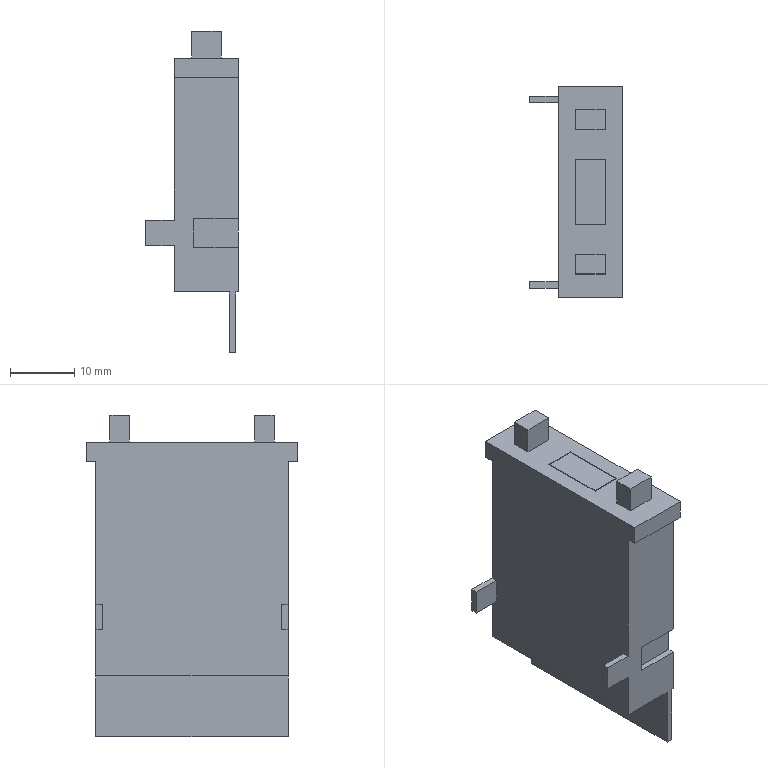Part | STEP file | A7PH_206_BASE | 1 solid | 50 faces | box 14.5 x 33 x 50.2 mm | volume 11412 mm3 | plane 50
STEP:
#1=CARTESIAN_POINT('',(-10.,-14.,-26.3));
#2=VERTEX_POINT('',#1);
#3=CARTESIAN_POINT('',(-10.,-15.,-26.3));
#4=VERTEX_POINT('',#3);
#5=CARTESIAN_POINT('',(-10.,-14.,-26.3));
#6=DIRECTION('',(0.,-1.,0.));
#7=VECTOR('',#6,1000.);
#8=LINE('',#5,#7);
#9=EDGE_CURVE('',#2,#4,#8,.T.);
#10=ORIENTED_EDGE('',*,*,#9,.F.);
#11=CARTESIAN_POINT('',(-10.,-14.,-22.3));
#12=VERTEX_POINT('',#11);
#13=CARTESIAN_POINT('',(-10.,-14.,-26.3));
#14=DIRECTION('',(0.,0.,-1.));
#15=VECTOR('',#14,1000.);
#16=LINE('',#13,#15);
#17=EDGE_CURVE('',#12,#2,#16,.T.);
#18=ORIENTED_EDGE('',*,*,#17,.F.);
#19=CARTESIAN_POINT('',(-10.,-15.,-22.3));
#20=VERTEX_POINT('',#19);
#21=CARTESIAN_POINT('',(-10.,-14.,-22.3));
#22=DIRECTION('',(0.,1.,0.));
#23=VECTOR('',#22,1000.);
#24=LINE('',#21,#23);
#25=EDGE_CURVE('',#20,#12,#24,.T.);
#26=ORIENTED_EDGE('',*,*,#25,.F.);
#27=CARTESIAN_POINT('',(-10.,-15.,0.));
#28=VERTEX_POINT('',#27);
#29=CARTESIAN_POINT('',(-10.,-15.,0.));
#30=DIRECTION('',(0.,0.,-1.));
#31=VECTOR('',#30,1000.);
#32=LINE('',#29,#31);
#33=EDGE_CURVE('',#28,#20,#32,.T.);
#34=ORIENTED_EDGE('',*,*,#33,.F.);
#35=CARTESIAN_POINT('',(-10.,-16.5,0.));
#36=VERTEX_POINT('',#35);
#37=CARTESIAN_POINT('',(-10.,-16.5,0.));
#38=DIRECTION('',(0.,1.,0.));
#39=VECTOR('',#38,1000.);
#40=LINE('',#37,#39);
#41=EDGE_CURVE('',#36,#28,#40,.T.);
#42=ORIENTED_EDGE('',*,*,#41,.F.);
#43=CARTESIAN_POINT('',(-10.,-16.5,3.));
#44=VERTEX_POINT('',#43);
#45=CARTESIAN_POINT('',(-10.,-16.5,3.));
#46=DIRECTION('',(0.,0.,-1.));
#47=VECTOR('',#46,1000.);
#48=LINE('',#45,#47);
#49=EDGE_CURVE('',#44,#36,#48,.T.);
#50=ORIENTED_EDGE('',*,*,#49,.F.);
#51=CARTESIAN_POINT('',(-10.,16.5,3.));
#52=VERTEX_POINT('',#51);
#53=CARTESIAN_POINT('',(-10.,16.5,3.));
#54=DIRECTION('',(0.,-1.,0.));
#55=VECTOR('',#54,1000.);
#56=LINE('',#53,#55);
#57=EDGE_CURVE('',#52,#44,#56,.T.);
#58=ORIENTED_EDGE('',*,*,#57,.F.);
#59=CARTESIAN_POINT('',(-10.,16.5,0.));
#60=VERTEX_POINT('',#59);
#61=CARTESIAN_POINT('',(-10.,16.5,0.));
#62=DIRECTION('',(0.,0.,1.));
#63=VECTOR('',#62,1000.);
#64=LINE('',#61,#63);
#65=EDGE_CURVE('',#60,#52,#64,.T.);
#66=ORIENTED_EDGE('',*,*,#65,.F.);
#67=CARTESIAN_POINT('',(-10.,15.,0.));
#68=VERTEX_POINT('',#67);
#69=CARTESIAN_POINT('',(-10.,15.,0.));
#70=DIRECTION('',(0.,1.,0.));
#71=VECTOR('',#70,1000.);
#72=LINE('',#69,#71);
#73=EDGE_CURVE('',#68,#60,#72,.T.);
#74=ORIENTED_EDGE('',*,*,#73,.F.);
#75=CARTESIAN_POINT('',(-10.,15.,-22.3));
#76=VERTEX_POINT('',#75);
#77=CARTESIAN_POINT('',(-10.,15.,0.));
#78=DIRECTION('',(0.,0.,1.));
#79=VECTOR('',#78,1000.);
#80=LINE('',#77,#79);
#81=EDGE_CURVE('',#76,#68,#80,.T.);
#82=ORIENTED_EDGE('',*,*,#81,.F.);
#83=CARTESIAN_POINT('',(-10.,14.,-22.3));
#84=VERTEX_POINT('',#83);
#85=CARTESIAN_POINT('',(-10.,15.,-22.3));
#86=DIRECTION('',(0.,1.,0.));
#87=VECTOR('',#86,1000.);
#88=LINE('',#85,#87);
#89=EDGE_CURVE('',#84,#76,#88,.T.);
#90=ORIENTED_EDGE('',*,*,#89,.F.);
#91=CARTESIAN_POINT('',(-10.,14.,-26.3));
#92=VERTEX_POINT('',#91);
#93=CARTESIAN_POINT('',(-10.,14.,-26.3));
#94=DIRECTION('',(0.,0.,1.));
#95=VECTOR('',#94,1000.);
#96=LINE('',#93,#95);
#97=EDGE_CURVE('',#92,#84,#96,.T.);
#98=ORIENTED_EDGE('',*,*,#97,.F.);
#99=CARTESIAN_POINT('',(-10.,15.,-26.3));
#100=VERTEX_POINT('',#99);
#101=CARTESIAN_POINT('',(-10.,15.,-26.3));
#102=DIRECTION('',(0.,-1.,0.));
#103=VECTOR('',#102,1000.);
#104=LINE('',#101,#103);
#105=EDGE_CURVE('',#100,#92,#104,.T.);
#106=ORIENTED_EDGE('',*,*,#105,.F.);
#107=CARTESIAN_POINT('',(-10.,15.,-33.5));
#108=VERTEX_POINT('',#107);
#109=CARTESIAN_POINT('',(-10.,15.,0.));
#110=DIRECTION('',(0.,0.,1.));
#111=VECTOR('',#110,1000.);
#112=LINE('',#109,#111);
#113=EDGE_CURVE('',#108,#100,#112,.T.);
#114=ORIENTED_EDGE('',*,*,#113,.F.);
#115=CARTESIAN_POINT('',(-10.,-15.,-33.5));
#116=VERTEX_POINT('',#115);
#117=CARTESIAN_POINT('',(-10.,15.,-33.5));
#118=DIRECTION('',(0.,1.,0.));
#119=VECTOR('',#118,1000.);
#120=LINE('',#117,#119);
#121=EDGE_CURVE('',#116,#108,#120,.T.);
#122=ORIENTED_EDGE('',*,*,#121,.F.);
#123=CARTESIAN_POINT('',(-10.,-15.,0.));
#124=DIRECTION('',(0.,0.,-1.));
#125=VECTOR('',#124,1000.);
#126=LINE('',#123,#125);
#127=EDGE_CURVE('',#4,#116,#126,.T.);
#128=ORIENTED_EDGE('',*,*,#127,.F.);
#129=EDGE_LOOP('',(#10,#18,#26,#34,#42,#50,#58,#66,#74,#82,#90,#98,#106,#114,#122,#128));
#130=FACE_OUTER_BOUND('',#129,.T.);
#131=CARTESIAN_POINT('',(-10.,16.5,0.));
#132=DIRECTION('',(1.,0.,0.));
#133=DIRECTION('',(0.,0.,-1.));
#134=AXIS2_PLACEMENT_3D('',#131,#132,#133);
#135=PLANE('',#134);
#136=ADVANCED_FACE('',(#130),#135,.F.);
#137=CARTESIAN_POINT('',(-1.4,15.,-33.5));
#138=VERTEX_POINT('',#137);
#139=CARTESIAN_POINT('',(-10.,15.,-33.5));
#140=DIRECTION('',(1.,0.,0.));
#141=VECTOR('',#140,1000.);
#142=LINE('',#139,#141);
#143=EDGE_CURVE('',#108,#138,#142,.T.);
#144=ORIENTED_EDGE('',*,*,#143,.T.);
#145=CARTESIAN_POINT('',(-1.4,-15.,-33.5));
#146=VERTEX_POINT('',#145);
#147=CARTESIAN_POINT('',(-1.4,24.552,-33.5));
#148=DIRECTION('',(0.,-1.,0.));
#149=VECTOR('',#148,1000.);
#150=LINE('',#147,#149);
#151=EDGE_CURVE('',#138,#146,#150,.T.);
#152=ORIENTED_EDGE('',*,*,#151,.T.);
#153=CARTESIAN_POINT('',(-10.,-15.,-33.5));
#154=DIRECTION('',(1.,0.,0.));
#155=VECTOR('',#154,1000.);
#156=LINE('',#153,#155);
#157=EDGE_CURVE('',#116,#146,#156,.T.);
#158=ORIENTED_EDGE('',*,*,#157,.F.);
#159=ORIENTED_EDGE('',*,*,#121,.T.);
#160=EDGE_LOOP('',(#144,#152,#158,#159));
#161=FACE_OUTER_BOUND('',#160,.T.);
#162=CARTESIAN_POINT('',(-10.,15.,-33.5));
#163=DIRECTION('',(0.,0.,-1.));
#164=DIRECTION('',(-1.,0.,0.));
#165=AXIS2_PLACEMENT_3D('',#162,#163,#164);
#166=PLANE('',#165);
#167=ADVANCED_FACE('',(#161),#166,.T.);
#168=CARTESIAN_POINT('',(-7.4,5.1,3.));
#169=VERTEX_POINT('',#168);
#170=CARTESIAN_POINT('',(-7.4,-5.1,3.));
#171=VERTEX_POINT('',#170);
#172=CARTESIAN_POINT('',(-7.4,5.,3.));
#173=DIRECTION('',(0.,-1.,0.));
#174=VECTOR('',#173,1000.);
#175=LINE('',#172,#174);
#176=EDGE_CURVE('',#169,#171,#175,.T.);
#177=ORIENTED_EDGE('',*,*,#176,.F.);
#178=CARTESIAN_POINT('',(-2.6,5.1,3.));
#179=VERTEX_POINT('',#178);
#180=CARTESIAN_POINT('',(-7.3,5.1,3.));
#181=DIRECTION('',(-1.,0.,0.));
#182=VECTOR('',#181,1000.);
#183=LINE('',#180,#182);
#184=EDGE_CURVE('',#179,#169,#183,.T.);
#185=ORIENTED_EDGE('',*,*,#184,.F.);
#186=CARTESIAN_POINT('',(-2.6,-5.1,3.));
#187=VERTEX_POINT('',#186);
#188=CARTESIAN_POINT('',(-2.6,5.,3.));
#189=DIRECTION('',(0.,1.,0.));
#190=VECTOR('',#189,1000.);
#191=LINE('',#188,#190);
#192=EDGE_CURVE('',#187,#179,#191,.T.);
#193=ORIENTED_EDGE('',*,*,#192,.F.);
#194=CARTESIAN_POINT('',(-7.3,-5.1,3.));
#195=DIRECTION('',(1.,0.,0.));
#196=VECTOR('',#195,1000.);
#197=LINE('',#194,#196);
#198=EDGE_CURVE('',#171,#187,#197,.T.);
#199=ORIENTED_EDGE('',*,*,#198,.F.);
#200=EDGE_LOOP('',(#177,#185,#193,#199));
#201=FACE_BOUND('',#200,.T.);
#202=CARTESIAN_POINT('',(-7.3,-12.8,3.));
#203=VERTEX_POINT('',#202);
#204=CARTESIAN_POINT('',(-7.3,-9.8,3.));
#205=VERTEX_POINT('',#204);
#206=CARTESIAN_POINT('',(-7.3,-12.8,3.));
#207=DIRECTION('',(0.,1.,0.));
#208=VECTOR('',#207,1000.);
#209=LINE('',#206,#208);
#210=EDGE_CURVE('',#203,#205,#209,.T.);
#211=ORIENTED_EDGE('',*,*,#210,.T.);
#212=CARTESIAN_POINT('',(-2.7,-9.8,3.));
#213=VERTEX_POINT('',#212);
#214=CARTESIAN_POINT('',(-7.3,-9.8,3.));
#215=DIRECTION('',(1.,0.,0.));
#216=VECTOR('',#215,1000.);
#217=LINE('',#214,#216);
#218=EDGE_CURVE('',#205,#213,#217,.T.);
#219=ORIENTED_EDGE('',*,*,#218,.T.);
#220=CARTESIAN_POINT('',(-2.7,-12.8,3.));
#221=VERTEX_POINT('',#220);
#222=CARTESIAN_POINT('',(-2.7,-12.8,3.));
#223=DIRECTION('',(0.,-1.,0.));
#224=VECTOR('',#223,1000.);
#225=LINE('',#222,#224);
#226=EDGE_CURVE('',#213,#221,#225,.T.);
#227=ORIENTED_EDGE('',*,*,#226,.T.);
#228=CARTESIAN_POINT('',(-7.3,-12.8,3.));
#229=DIRECTION('',(-1.,0.,0.));
#230=VECTOR('',#229,1000.);
#231=LINE('',#228,#230);
#232=EDGE_CURVE('',#221,#203,#231,.T.);
#233=ORIENTED_EDGE('',*,*,#232,.T.);
#234=EDGE_LOOP('',(#211,#219,#227,#233));
#235=FACE_BOUND('',#234,.T.);
#236=CARTESIAN_POINT('',(0.,16.5,3.));
#237=VERTEX_POINT('',#236);
#238=CARTESIAN_POINT('',(0.,-16.5,3.));
#239=VERTEX_POINT('',#238);
#240=CARTESIAN_POINT('',(0.,16.5,3.));
#241=DIRECTION('',(0.,-1.,0.));
#242=VECTOR('',#241,1000.);
#243=LINE('',#240,#242);
#244=EDGE_CURVE('',#237,#239,#243,.T.);
#245=ORIENTED_EDGE('',*,*,#244,.F.);
#246=CARTESIAN_POINT('',(-10.,16.5,3.));
#247=DIRECTION('',(1.,0.,0.));
#248=VECTOR('',#247,1000.);
#249=LINE('',#246,#248);
#250=EDGE_CURVE('',#52,#237,#249,.T.);
#251=ORIENTED_EDGE('',*,*,#250,.F.);
#252=ORIENTED_EDGE('',*,*,#57,.T.);
#253=CARTESIAN_POINT('',(-10.,-16.5,3.));
#254=DIRECTION('',(1.,0.,0.));
#255=VECTOR('',#254,1000.);
#256=LINE('',#253,#255);
#257=EDGE_CURVE('',#44,#239,#256,.T.);
#258=ORIENTED_EDGE('',*,*,#257,.T.);
#259=EDGE_LOOP('',(#245,#251,#252,#258));
#260=FACE_OUTER_BOUND('',#259,.T.);
#261=CARTESIAN_POINT('',(-7.3,9.8,3.));
#262=VERTEX_POINT('',#261);
#263=CARTESIAN_POINT('',(-2.7,9.8,3.));
#264=VERTEX_POINT('',#263);
#265=CARTESIAN_POINT('',(-7.3,9.8,3.));
#266=DIRECTION('',(1.,0.,0.));
#267=VECTOR('',#266,1000.);
#268=LINE('',#265,#267);
#269=EDGE_CURVE('',#262,#264,#268,.T.);
#270=ORIENTED_EDGE('',*,*,#269,.F.);
#271=CARTESIAN_POINT('',(-7.3,12.8,3.));
#272=VERTEX_POINT('',#271);
#273=CARTESIAN_POINT('',(-7.3,12.8,3.));
#274=DIRECTION('',(0.,-1.,0.));
#275=VECTOR('',#274,1000.);
#276=LINE('',#273,#275);
#277=EDGE_CURVE('',#272,#262,#276,.T.);
#278=ORIENTED_EDGE('',*,*,#277,.F.);
#279=CARTESIAN_POINT('',(-2.7,12.8,3.));
#280=VERTEX_POINT('',#279);
#281=CARTESIAN_POINT('',(-7.3,12.8,3.));
#282=DIRECTION('',(-1.,0.,0.));
#283=VECTOR('',#282,1000.);
#284=LINE('',#281,#283);
#285=EDGE_CURVE('',#280,#272,#284,.T.);
#286=ORIENTED_EDGE('',*,*,#285,.F.);
#287=CARTESIAN_POINT('',(-2.7,12.8,3.));
#288=DIRECTION('',(0.,1.,0.));
#289=VECTOR('',#288,1000.);
#290=LINE('',#287,#289);
#291=EDGE_CURVE('',#264,#280,#290,.T.);
#292=ORIENTED_EDGE('',*,*,#291,.F.);
#293=EDGE_LOOP('',(#270,#278,#286,#292));
#294=FACE_BOUND('',#293,.T.);
#295=CARTESIAN_POINT('',(-10.,16.5,3.));
#296=DIRECTION('',(0.,0.,1.));
#297=DIRECTION('',(1.,0.,0.));
#298=AXIS2_PLACEMENT_3D('',#295,#296,#297);
#299=PLANE('',#298);
#300=ADVANCED_FACE('',(#201,#235,#260,#294),#299,.T.);
#301=CARTESIAN_POINT('',(0.,15.,0.));
#302=VERTEX_POINT('',#301);
#303=CARTESIAN_POINT('',(0.,16.5,0.));
#304=VERTEX_POINT('',#303);
#305=CARTESIAN_POINT('',(0.,15.,0.));
#306=DIRECTION('',(0.,1.,0.));
#307=VECTOR('',#306,1000.);
#308=LINE('',#305,#307);
#309=EDGE_CURVE('',#302,#304,#308,.T.);
#310=ORIENTED_EDGE('',*,*,#309,.F.);
#311=CARTESIAN_POINT('',(-10.,15.,0.));
#312=DIRECTION('',(1.,0.,0.));
#313=VECTOR('',#312,1000.);
#314=LINE('',#311,#313);
#315=EDGE_CURVE('',#68,#302,#314,.T.);
#316=ORIENTED_EDGE('',*,*,#315,.F.);
#317=ORIENTED_EDGE('',*,*,#73,.T.);
#318=CARTESIAN_POINT('',(-10.,16.5,0.));
#319=DIRECTION('',(1.,0.,0.));
#320=VECTOR('',#319,1000.);
#321=LINE('',#318,#320);
#322=EDGE_CURVE('',#60,#304,#321,.T.);
#323=ORIENTED_EDGE('',*,*,#322,.T.);
#324=EDGE_LOOP('',(#310,#316,#317,#323));
#325=FACE_OUTER_BOUND('',#324,.T.);
#326=CARTESIAN_POINT('',(-10.,15.,0.));
#327=DIRECTION('',(0.,0.,-1.));
#328=DIRECTION('',(0.,1.,0.));
#329=AXIS2_PLACEMENT_3D('',#326,#327,#328);
#330=PLANE('',#329);
#331=ADVANCED_FACE('',(#325),#330,.T.);
#332=CARTESIAN_POINT('',(-7.,15.,-22.1));
#333=VERTEX_POINT('',#332);
#334=CARTESIAN_POINT('',(0.,15.,-22.1));
#335=VERTEX_POINT('',#334);
#336=CARTESIAN_POINT('',(-7.,15.,-22.1));
#337=DIRECTION('',(1.,0.,0.));
#338=VECTOR('',#337,1000.);
#339=LINE('',#336,#338);
#340=EDGE_CURVE('',#333,#335,#339,.T.);
#341=ORIENTED_EDGE('',*,*,#340,.F.);
#342=CARTESIAN_POINT('',(-7.,15.,-26.5));
#343=VERTEX_POINT('',#342);
#344=CARTESIAN_POINT('',(-7.,15.,-22.1));
#345=DIRECTION('',(0.,0.,1.));
#346=VECTOR('',#345,1000.);
#347=LINE('',#344,#346);
#348=EDGE_CURVE('',#343,#333,#347,.T.);
#349=ORIENTED_EDGE('',*,*,#348,.F.);
#350=CARTESIAN_POINT('',(0.,15.,-26.5));
#351=VERTEX_POINT('',#350);
#352=CARTESIAN_POINT('',(-7.,15.,-26.5));
#353=DIRECTION('',(1.,0.,0.));
#354=VECTOR('',#353,1000.);
#355=LINE('',#352,#354);
#356=EDGE_CURVE('',#343,#351,#355,.T.);
#357=ORIENTED_EDGE('',*,*,#356,.T.);
#358=CARTESIAN_POINT('',(0.,15.,-33.5));
#359=VERTEX_POINT('',#358);
#360=CARTESIAN_POINT('',(0.,15.,0.));
#361=DIRECTION('',(0.,0.,1.));
#362=VECTOR('',#361,1000.);
#363=LINE('',#360,#362);
#364=EDGE_CURVE('',#359,#351,#363,.T.);
#365=ORIENTED_EDGE('',*,*,#364,.F.);
#366=CARTESIAN_POINT('',(-0.4,15.,-33.5));
#367=VERTEX_POINT('',#366);
#368=CARTESIAN_POINT('',(-10.,15.,-33.5));
#369=DIRECTION('',(1.,0.,0.));
#370=VECTOR('',#369,1000.);
#371=LINE('',#368,#370);
#372=EDGE_CURVE('',#367,#359,#371,.T.);
#373=ORIENTED_EDGE('',*,*,#372,.F.);
#374=CARTESIAN_POINT('',(-0.4,15.,-43.));
#375=VERTEX_POINT('',#374);
#376=CARTESIAN_POINT('',(-0.4,15.,-33.5));
#377=DIRECTION('',(0.,0.,1.));
#378=VECTOR('',#377,1000.);
#379=LINE('',#376,#378);
#380=EDGE_CURVE('',#375,#367,#379,.T.);
#381=ORIENTED_EDGE('',*,*,#380,.F.);
#382=CARTESIAN_POINT('',(-1.4,15.,-43.));
#383=VERTEX_POINT('',#382);
#384=CARTESIAN_POINT('',(-0.4,15.,-43.));
#385=DIRECTION('',(1.,0.,0.));
#386=VECTOR('',#385,1000.);
#387=LINE('',#384,#386);
#388=EDGE_CURVE('',#383,#375,#387,.T.);
#389=ORIENTED_EDGE('',*,*,#388,.F.);
#390=CARTESIAN_POINT('',(-1.4,15.,-33.5));
#391=DIRECTION('',(0.,0.,-1.));
#392=VECTOR('',#391,1000.);
#393=LINE('',#390,#392);
#394=EDGE_CURVE('',#138,#383,#393,.T.);
#395=ORIENTED_EDGE('',*,*,#394,.F.);
#396=ORIENTED_EDGE('',*,*,#143,.F.);
#397=ORIENTED_EDGE('',*,*,#113,.T.);
#398=CARTESIAN_POINT('',(-14.5,15.,-26.3));
#399=VERTEX_POINT('',#398);
#400=CARTESIAN_POINT('',(-14.5,15.,-26.3));
#401=DIRECTION('',(1.,0.,0.));
#402=VECTOR('',#401,1000.);
#403=LINE('',#400,#402);
#404=EDGE_CURVE('',#399,#100,#403,.T.);
#405=ORIENTED_EDGE('',*,*,#404,.F.);
#406=CARTESIAN_POINT('',(-14.5,15.,-22.3));
#407=VERTEX_POINT('',#406);
#408=CARTESIAN_POINT('',(-14.5,15.,-26.3));
#409=DIRECTION('',(0.,0.,-1.));
#410=VECTOR('',#409,1000.);
#411=LINE('',#408,#410);
#412=EDGE_CURVE('',#407,#399,#411,.T.);
#413=ORIENTED_EDGE('',*,*,#412,.F.);
#414=CARTESIAN_POINT('',(-14.5,15.,-22.3));
#415=DIRECTION('',(1.,0.,0.));
#416=VECTOR('',#415,1000.);
#417=LINE('',#414,#416);
#418=EDGE_CURVE('',#407,#76,#417,.T.);
#419=ORIENTED_EDGE('',*,*,#418,.T.);
#420=ORIENTED_EDGE('',*,*,#81,.T.);
#421=ORIENTED_EDGE('',*,*,#315,.T.);
#422=CARTESIAN_POINT('',(0.,15.,0.));
#423=DIRECTION('',(0.,0.,1.));
#424=VECTOR('',#423,1000.);
#425=LINE('',#422,#424);
#426=EDGE_CURVE('',#335,#302,#425,.T.);
#427=ORIENTED_EDGE('',*,*,#426,.F.);
#428=EDGE_LOOP('',(#341,#349,#357,#365,#373,#381,#389,#395,#396,#397,#405,#413,#419,#420,#421,#427));
#429=FACE_OUTER_BOUND('',#428,.T.);
#430=CARTESIAN_POINT('',(-10.,15.,0.));
#431=DIRECTION('',(0.,1.,0.));
#432=DIRECTION('',(0.,0.,1.));
#433=AXIS2_PLACEMENT_3D('',#430,#431,#432);
#434=PLANE('',#433);
#435=ADVANCED_FACE('',(#429),#434,.T.);
#436=CARTESIAN_POINT('',(-0.4,-15.,-33.5));
#437=VERTEX_POINT('',#436);
#438=CARTESIAN_POINT('',(-0.4,24.552,-33.5));
#439=DIRECTION('',(0.,-1.,0.));
#440=VECTOR('',#439,1000.);
#441=LINE('',#438,#440);
#442=EDGE_CURVE('',#367,#437,#441,.T.);
#443=ORIENTED_EDGE('',*,*,#442,.F.);
#444=ORIENTED_EDGE('',*,*,#372,.T.);
#445=CARTESIAN_POINT('',(0.,-15.,-33.5));
#446=VERTEX_POINT('',#445);
#447=CARTESIAN_POINT('',(0.,15.,-33.5));
#448=DIRECTION('',(0.,1.,0.));
#449=VECTOR('',#448,1000.);
#450=LINE('',#447,#449);
#451=EDGE_CURVE('',#446,#359,#450,.T.);
#452=ORIENTED_EDGE('',*,*,#451,.F.);
#453=CARTESIAN_POINT('',(-10.,-15.,-33.5));
#454=DIRECTION('',(1.,0.,0.));
#455=VECTOR('',#454,1000.);
#456=LINE('',#453,#455);
#457=EDGE_CURVE('',#437,#446,#456,.T.);
#458=ORIENTED_EDGE('',*,*,#457,.F.);
#459=EDGE_LOOP('',(#443,#444,#452,#458));
#460=FACE_OUTER_BOUND('',#459,.T.);
#461=CARTESIAN_POINT('',(-10.,15.,-33.5));
#462=DIRECTION('',(0.,0.,-1.));
#463=DIRECTION('',(-1.,0.,0.));
#464=AXIS2_PLACEMENT_3D('',#461,#462,#463);
#465=PLANE('',#464);
#466=ADVANCED_FACE('',(#460),#465,.T.);
#467=CARTESIAN_POINT('',(-7.,-15.,-22.1));
#468=VERTEX_POINT('',#467);
#469=CARTESIAN_POINT('',(0.,-15.,-22.1));
#470=VERTEX_POINT('',#469);
#471=CARTESIAN_POINT('',(-7.,-15.,-22.1));
#472=DIRECTION('',(1.,0.,0.));
#473=VECTOR('',#472,1000.);
#474=LINE('',#471,#473);
#475=EDGE_CURVE('',#468,#470,#474,.T.);
#476=ORIENTED_EDGE('',*,*,#475,.T.);
#477=CARTESIAN_POINT('',(0.,-15.,0.));
#478=VERTEX_POINT('',#477);
#479=CARTESIAN_POINT('',(0.,-15.,0.));
#480=DIRECTION('',(0.,0.,-1.));
#481=VECTOR('',#480,1000.);
#482=LINE('',#479,#481);
#483=EDGE_CURVE('',#478,#470,#482,.T.);
#484=ORIENTED_EDGE('',*,*,#483,.F.);
#485=CARTESIAN_POINT('',(-10.,-15.,0.));
#486=DIRECTION('',(1.,0.,0.));
#487=VECTOR('',#486,1000.);
#488=LINE('',#485,#487);
#489=EDGE_CURVE('',#28,#478,#488,.T.);
#490=ORIENTED_EDGE('',*,*,#489,.F.);
#491=ORIENTED_EDGE('',*,*,#33,.T.);
#492=CARTESIAN_POINT('',(-14.5,-15.,-22.3));
#493=VERTEX_POINT('',#492);
#494=CARTESIAN_POINT('',(-14.5,-15.,-22.3));
#495=DIRECTION('',(1.,0.,0.));
#496=VECTOR('',#495,1000.);
#497=LINE('',#494,#496);
#498=EDGE_CURVE('',#493,#20,#497,.T.);
#499=ORIENTED_EDGE('',*,*,#498,.F.);
#500=CARTESIAN_POINT('',(-14.5,-15.,-26.3));
#501=VERTEX_POINT('',#500);
#502=CARTESIAN_POINT('',(-14.5,-15.,-26.3));
#503=DIRECTION('',(0.,0.,1.));
#504=VECTOR('',#503,1000.);
#505=LINE('',#502,#504);
#506=EDGE_CURVE('',#501,#493,#505,.T.);
#507=ORIENTED_EDGE('',*,*,#506,.F.);
#508=CARTESIAN_POINT('',(-14.5,-15.,-26.3));
#509=DIRECTION('',(1.,0.,0.));
#510=VECTOR('',#509,1000.);
#511=LINE('',#508,#510);
#512=EDGE_CURVE('',#501,#4,#511,.T.);
#513=ORIENTED_EDGE('',*,*,#512,.T.);
#514=ORIENTED_EDGE('',*,*,#127,.T.);
#515=ORIENTED_EDGE('',*,*,#157,.T.);
#516=CARTESIAN_POINT('',(-1.4,-15.,-43.));
#517=VERTEX_POINT('',#516);
#518=CARTESIAN_POINT('',(-1.4,-15.,-33.5));
#519=DIRECTION('',(0.,0.,-1.));
#520=VECTOR('',#519,1000.);
#521=LINE('',#518,#520);
#522=EDGE_CURVE('',#146,#517,#521,.T.);
#523=ORIENTED_EDGE('',*,*,#522,.T.);
#524=CARTESIAN_POINT('',(-0.4,-15.,-43.));
#525=VERTEX_POINT('',#524);
#526=CARTESIAN_POINT('',(-0.4,-15.,-43.));
#527=DIRECTION('',(1.,0.,0.));
#528=VECTOR('',#527,1000.);
#529=LINE('',#526,#528);
#530=EDGE_CURVE('',#517,#525,#529,.T.);
#531=ORIENTED_EDGE('',*,*,#530,.T.);
#532=CARTESIAN_POINT('',(-0.4,-15.,-33.5));
#533=DIRECTION('',(0.,0.,1.));
#534=VECTOR('',#533,1000.);
#535=LINE('',#532,#534);
#536=EDGE_CURVE('',#525,#437,#535,.T.);
#537=ORIENTED_EDGE('',*,*,#536,.T.);
#538=ORIENTED_EDGE('',*,*,#457,.T.);
#539=CARTESIAN_POINT('',(0.,-15.,-26.5));
#540=VERTEX_POINT('',#539);
#541=CARTESIAN_POINT('',(0.,-15.,0.));
#542=DIRECTION('',(0.,0.,-1.));
#543=VECTOR('',#542,1000.);
#544=LINE('',#541,#543);
#545=EDGE_CURVE('',#540,#446,#544,.T.);
#546=ORIENTED_EDGE('',*,*,#545,.F.);
#547=CARTESIAN_POINT('',(-7.,-15.,-26.5));
#548=VERTEX_POINT('',#547);
#549=CARTESIAN_POINT('',(-7.,-15.,-26.5));
#550=DIRECTION('',(1.,0.,0.));
#551=VECTOR('',#550,1000.);
#552=LINE('',#549,#551);
#553=EDGE_CURVE('',#548,#540,#552,.T.);
#554=ORIENTED_EDGE('',*,*,#553,.F.);
#555=CARTESIAN_POINT('',(-7.,-15.,-22.1));
#556=DIRECTION('',(0.,0.,-1.));
#557=VECTOR('',#556,1000.);
#558=LINE('',#555,#557);
#559=EDGE_CURVE('',#468,#548,#558,.T.);
#560=ORIENTED_EDGE('',*,*,#559,.F.);
#561=EDGE_LOOP('',(#476,#484,#490,#491,#499,#507,#513,#514,#515,#523,#531,#537,#538,#546,#554,#560));
#562=FACE_OUTER_BOUND('',#561,.T.);
#563=CARTESIAN_POINT('',(-10.,-15.,0.));
#564=DIRECTION('',(0.,-1.,0.));
#565=DIRECTION('',(0.,0.,-1.));
#566=AXIS2_PLACEMENT_3D('',#563,#564,#565);
#567=PLANE('',#566);
#568=ADVANCED_FACE('',(#562),#567,.T.);
#569=CARTESIAN_POINT('',(0.,-16.5,0.));
#570=VERTEX_POINT('',#569);
#571=CARTESIAN_POINT('',(0.,-16.5,0.));
#572=DIRECTION('',(0.,1.,0.));
#573=VECTOR('',#572,1000.);
#574=LINE('',#571,#573);
#575=EDGE_CURVE('',#570,#478,#574,.T.);
#576=ORIENTED_EDGE('',*,*,#575,.F.);
#577=CARTESIAN_POINT('',(-10.,-16.5,0.));
#578=DIRECTION('',(1.,0.,0.));
#579=VECTOR('',#578,1000.);
#580=LINE('',#577,#579);
#581=EDGE_CURVE('',#36,#570,#580,.T.);
#582=ORIENTED_EDGE('',*,*,#581,.F.);
#583=ORIENTED_EDGE('',*,*,#41,.T.);
#584=ORIENTED_EDGE('',*,*,#489,.T.);
#585=EDGE_LOOP('',(#576,#582,#583,#584));
#586=FACE_OUTER_BOUND('',#585,.T.);
#587=CARTESIAN_POINT('',(-10.,-16.5,0.));
#588=DIRECTION('',(0.,0.,-1.));
#589=DIRECTION('',(-1.,0.,0.));
#590=AXIS2_PLACEMENT_3D('',#587,#588,#589);
#591=PLANE('',#590);
#592=ADVANCED_FACE('',(#586),#591,.T.);
#593=CARTESIAN_POINT('',(0.,-16.5,3.));
#594=DIRECTION('',(0.,0.,-1.));
#595=VECTOR('',#594,1000.);
#596=LINE('',#593,#595);
#597=EDGE_CURVE('',#239,#570,#596,.T.);
#598=ORIENTED_EDGE('',*,*,#597,.F.);
#599=ORIENTED_EDGE('',*,*,#257,.F.);
#600=ORIENTED_EDGE('',*,*,#49,.T.);
#601=ORIENTED_EDGE('',*,*,#581,.T.);
#602=EDGE_LOOP('',(#598,#599,#600,#601));
#603=FACE_OUTER_BOUND('',#602,.T.);
#604=CARTESIAN_POINT('',(-10.,-16.5,3.));
#605=DIRECTION('',(0.,-1.,0.));
#606=DIRECTION('',(0.,0.,-1.));
#607=AXIS2_PLACEMENT_3D('',#604,#605,#606);
#608=PLANE('',#607);
#609=ADVANCED_FACE('',(#603),#608,.T.);
#610=CARTESIAN_POINT('',(0.,16.5,0.));
#611=DIRECTION('',(0.,0.,1.));
#612=VECTOR('',#611,1000.);
#613=LINE('',#610,#612);
#614=EDGE_CURVE('',#304,#237,#613,.T.);
#615=ORIENTED_EDGE('',*,*,#614,.F.);
#616=ORIENTED_EDGE('',*,*,#322,.F.);
#617=ORIENTED_EDGE('',*,*,#65,.T.);
#618=ORIENTED_EDGE('',*,*,#250,.T.);
#619=EDGE_LOOP('',(#615,#616,#617,#618));
#620=FACE_OUTER_BOUND('',#619,.T.);
#621=CARTESIAN_POINT('',(-10.,16.5,0.));
#622=DIRECTION('',(0.,1.,0.));
#623=DIRECTION('',(0.,0.,1.));
#624=AXIS2_PLACEMENT_3D('',#621,#622,#623);
#625=PLANE('',#624);
#626=ADVANCED_FACE('',(#620),#625,.T.);
#627=CARTESIAN_POINT('',(0.,-14.,-22.1));
#628=VERTEX_POINT('',#627);
#629=CARTESIAN_POINT('',(0.,-15.,-22.1));
#630=DIRECTION('',(0.,-1.,0.));
#631=VECTOR('',#630,1000.);
#632=LINE('',#629,#631);
#633=EDGE_CURVE('',#628,#470,#632,.T.);
#634=ORIENTED_EDGE('',*,*,#633,.F.);
#635=CARTESIAN_POINT('',(0.,-14.,-26.5));
#636=VERTEX_POINT('',#635);
#637=CARTESIAN_POINT('',(0.,-14.,-22.1));
#638=DIRECTION('',(0.,0.,1.));
#639=VECTOR('',#638,1000.);
#640=LINE('',#637,#639);
#641=EDGE_CURVE('',#636,#628,#640,.T.);
#642=ORIENTED_EDGE('',*,*,#641,.F.);
#643=CARTESIAN_POINT('',(0.,-15.,-26.5));
#644=DIRECTION('',(0.,1.,0.));
#645=VECTOR('',#644,1000.);
#646=LINE('',#643,#645);
#647=EDGE_CURVE('',#540,#636,#646,.T.);
#648=ORIENTED_EDGE('',*,*,#647,.F.);
#649=ORIENTED_EDGE('',*,*,#545,.T.);
#650=ORIENTED_EDGE('',*,*,#451,.T.);
#651=ORIENTED_EDGE('',*,*,#364,.T.);
#652=CARTESIAN_POINT('',(0.,14.,-26.5));
#653=VERTEX_POINT('',#652);
#654=CARTESIAN_POINT('',(0.,15.,-26.5));
#655=DIRECTION('',(0.,1.,0.));
#656=VECTOR('',#655,1000.);
#657=LINE('',#654,#656);
#658=EDGE_CURVE('',#653,#351,#657,.T.);
#659=ORIENTED_EDGE('',*,*,#658,.F.);
#660=CARTESIAN_POINT('',(0.,14.,-22.1));
#661=VERTEX_POINT('',#660);
#662=CARTESIAN_POINT('',(0.,14.,-22.1));
#663=DIRECTION('',(0.,0.,-1.));
#664=VECTOR('',#663,1000.);
#665=LINE('',#662,#664);
#666=EDGE_CURVE('',#661,#653,#665,.T.);
#667=ORIENTED_EDGE('',*,*,#666,.F.);
#668=CARTESIAN_POINT('',(0.,15.,-22.1));
#669=DIRECTION('',(0.,-1.,0.));
#670=VECTOR('',#669,1000.);
#671=LINE('',#668,#670);
#672=EDGE_CURVE('',#335,#661,#671,.T.);
#673=ORIENTED_EDGE('',*,*,#672,.F.);
#674=ORIENTED_EDGE('',*,*,#426,.T.);
#675=ORIENTED_EDGE('',*,*,#309,.T.);
#676=ORIENTED_EDGE('',*,*,#614,.T.);
#677=ORIENTED_EDGE('',*,*,#244,.T.);
#678=ORIENTED_EDGE('',*,*,#597,.T.);
#679=ORIENTED_EDGE('',*,*,#575,.T.);
#680=ORIENTED_EDGE('',*,*,#483,.T.);
#681=EDGE_LOOP('',(#634,#642,#648,#649,#650,#651,#659,#667,#673,#674,#675,#676,#677,#678,#679,#680));
#682=FACE_OUTER_BOUND('',#681,.T.);
#683=CARTESIAN_POINT('',(0.,16.5,0.));
#684=DIRECTION('',(1.,0.,0.));
#685=DIRECTION('',(0.,0.,-1.));
#686=AXIS2_PLACEMENT_3D('',#683,#684,#685);
#687=PLANE('',#686);
#688=ADVANCED_FACE('',(#682),#687,.T.);
#689=ORIENTED_EDGE('',*,*,#277,.T.);
#690=CARTESIAN_POINT('',(-7.3,9.8,7.2));
#691=VERTEX_POINT('',#690);
#692=CARTESIAN_POINT('',(-7.3,9.8,7.2));
#693=DIRECTION('',(0.,0.,-1.));
#694=VECTOR('',#693,1000.);
#695=LINE('',#692,#694);
#696=EDGE_CURVE('',#691,#262,#695,.T.);
#697=ORIENTED_EDGE('',*,*,#696,.F.);
#698=CARTESIAN_POINT('',(-7.3,12.8,7.2));
#699=VERTEX_POINT('',#698);
#700=CARTESIAN_POINT('',(-7.3,12.8,7.2));
#701=DIRECTION('',(0.,-1.,0.));
#702=VECTOR('',#701,1000.);
#703=LINE('',#700,#702);
#704=EDGE_CURVE('',#699,#691,#703,.T.);
#705=ORIENTED_EDGE('',*,*,#704,.F.);
#706=CARTESIAN_POINT('',(-7.3,12.8,7.2));
#707=DIRECTION('',(0.,0.,-1.));
#708=VECTOR('',#707,1000.);
#709=LINE('',#706,#708);
#710=EDGE_CURVE('',#699,#272,#709,.T.);
#711=ORIENTED_EDGE('',*,*,#710,.T.);
#712=EDGE_LOOP('',(#689,#697,#705,#711));
#713=FACE_OUTER_BOUND('',#712,.T.);
#714=CARTESIAN_POINT('',(-7.3,12.8,7.2));
#715=DIRECTION('',(1.,0.,0.));
#716=DIRECTION('',(0.,1.,0.));
#717=AXIS2_PLACEMENT_3D('',#714,#715,#716);
#718=PLANE('',#717);
#719=ADVANCED_FACE('',(#713),#718,.F.);
#720=ORIENTED_EDGE('',*,*,#269,.T.);
#721=CARTESIAN_POINT('',(-2.7,9.8,7.2));
#722=VERTEX_POINT('',#721);
#723=CARTESIAN_POINT('',(-2.7,9.8,7.2));
#724=DIRECTION('',(0.,0.,-1.));
#725=VECTOR('',#724,1000.);
#726=LINE('',#723,#725);
#727=EDGE_CURVE('',#722,#264,#726,.T.);
#728=ORIENTED_EDGE('',*,*,#727,.F.);
#729=CARTESIAN_POINT('',(-7.3,9.8,7.2));
#730=DIRECTION('',(1.,0.,0.));
#731=VECTOR('',#730,1000.);
#732=LINE('',#729,#731);
#733=EDGE_CURVE('',#691,#722,#732,.T.);
#734=ORIENTED_EDGE('',*,*,#733,.F.);
#735=ORIENTED_EDGE('',*,*,#696,.T.);
#736=EDGE_LOOP('',(#720,#728,#734,#735));
#737=FACE_OUTER_BOUND('',#736,.T.);
#738=CARTESIAN_POINT('',(-7.3,9.8,7.2));
#739=DIRECTION('',(0.,1.,0.));
#740=DIRECTION('',(0.,0.,1.));
#741=AXIS2_PLACEMENT_3D('',#738,#739,#740);
#742=PLANE('',#741);
#743=ADVANCED_FACE('',(#737),#742,.F.);
#744=ORIENTED_EDGE('',*,*,#291,.T.);
#745=CARTESIAN_POINT('',(-2.7,12.8,7.2));
#746=VERTEX_POINT('',#745);
#747=CARTESIAN_POINT('',(-2.7,12.8,7.2));
#748=DIRECTION('',(0.,0.,-1.));
#749=VECTOR('',#748,1000.);
#750=LINE('',#747,#749);
#751=EDGE_CURVE('',#746,#280,#750,.T.);
#752=ORIENTED_EDGE('',*,*,#751,.F.);
#753=CARTESIAN_POINT('',(-2.7,12.8,7.2));
#754=DIRECTION('',(0.,1.,0.));
#755=VECTOR('',#754,1000.);
#756=LINE('',#753,#755);
#757=EDGE_CURVE('',#722,#746,#756,.T.);
#758=ORIENTED_EDGE('',*,*,#757,.F.);
#759=ORIENTED_EDGE('',*,*,#727,.T.);
#760=EDGE_LOOP('',(#744,#752,#758,#759));
#761=FACE_OUTER_BOUND('',#760,.T.);
#762=CARTESIAN_POINT('',(-2.7,12.8,7.2));
#763=DIRECTION('',(-1.,0.,0.));
#764=DIRECTION('',(0.,-1.,0.));
#765=AXIS2_PLACEMENT_3D('',#762,#763,#764);
#766=PLANE('',#765);
#767=ADVANCED_FACE('',(#761),#766,.F.);
#768=ORIENTED_EDGE('',*,*,#285,.T.);
#769=ORIENTED_EDGE('',*,*,#710,.F.);
#770=CARTESIAN_POINT('',(-7.3,12.8,7.2));
#771=DIRECTION('',(-1.,0.,0.));
#772=VECTOR('',#771,1000.);
#773=LINE('',#770,#772);
#774=EDGE_CURVE('',#746,#699,#773,.T.);
#775=ORIENTED_EDGE('',*,*,#774,.F.);
#776=ORIENTED_EDGE('',*,*,#751,.T.);
#777=EDGE_LOOP('',(#768,#769,#775,#776));
#778=FACE_OUTER_BOUND('',#777,.T.);
#779=CARTESIAN_POINT('',(-7.3,12.8,7.2));
#780=DIRECTION('',(0.,-1.,0.));
#781=DIRECTION('',(1.,0.,0.));
#782=AXIS2_PLACEMENT_3D('',#779,#780,#781);
#783=PLANE('',#782);
#784=ADVANCED_FACE('',(#778),#783,.F.);
#785=ORIENTED_EDGE('',*,*,#704,.T.);
#786=ORIENTED_EDGE('',*,*,#733,.T.);
#787=ORIENTED_EDGE('',*,*,#757,.T.);
#788=ORIENTED_EDGE('',*,*,#774,.T.);
#789=EDGE_LOOP('',(#785,#786,#787,#788));
#790=FACE_OUTER_BOUND('',#789,.T.);
#791=CARTESIAN_POINT('',(-7.3,9.8,7.2));
#792=DIRECTION('',(0.,0.,1.));
#793=DIRECTION('',(1.,0.,0.));
#794=AXIS2_PLACEMENT_3D('',#791,#792,#793);
#795=PLANE('',#794);
#796=ADVANCED_FACE('',(#790),#795,.T.);
#797=ORIENTED_EDGE('',*,*,#210,.F.);
#798=CARTESIAN_POINT('',(-7.3,-12.8,7.2));
#799=VERTEX_POINT('',#798);
#800=CARTESIAN_POINT('',(-7.3,-12.8,7.2));
#801=DIRECTION('',(0.,0.,-1.));
#802=VECTOR('',#801,1000.);
#803=LINE('',#800,#802);
#804=EDGE_CURVE('',#799,#203,#803,.T.);
#805=ORIENTED_EDGE('',*,*,#804,.F.);
#806=CARTESIAN_POINT('',(-7.3,-9.8,7.2));
#807=VERTEX_POINT('',#806);
#808=CARTESIAN_POINT('',(-7.3,-12.8,7.2));
#809=DIRECTION('',(0.,1.,0.));
#810=VECTOR('',#809,1000.);
#811=LINE('',#808,#810);
#812=EDGE_CURVE('',#799,#807,#811,.T.);
#813=ORIENTED_EDGE('',*,*,#812,.T.);
#814=CARTESIAN_POINT('',(-7.3,-9.8,7.2));
#815=DIRECTION('',(0.,0.,-1.));
#816=VECTOR('',#815,1000.);
#817=LINE('',#814,#816);
#818=EDGE_CURVE('',#807,#205,#817,.T.);
#819=ORIENTED_EDGE('',*,*,#818,.T.);
#820=EDGE_LOOP('',(#797,#805,#813,#819));
#821=FACE_OUTER_BOUND('',#820,.T.);
#822=CARTESIAN_POINT('',(-7.3,-12.8,7.2));
#823=DIRECTION('',(-1.,0.,0.));
#824=DIRECTION('',(0.,-1.,0.));
#825=AXIS2_PLACEMENT_3D('',#822,#823,#824);
#826=PLANE('',#825);
#827=ADVANCED_FACE('',(#821),#826,.T.);
#828=ORIENTED_EDGE('',*,*,#232,.F.);
#829=CARTESIAN_POINT('',(-2.7,-12.8,7.2));
#830=VERTEX_POINT('',#829);
#831=CARTESIAN_POINT('',(-2.7,-12.8,7.2));
#832=DIRECTION('',(0.,0.,-1.));
#833=VECTOR('',#832,1000.);
#834=LINE('',#831,#833);
#835=EDGE_CURVE('',#830,#221,#834,.T.);
#836=ORIENTED_EDGE('',*,*,#835,.F.);
#837=CARTESIAN_POINT('',(-7.3,-12.8,7.2));
#838=DIRECTION('',(-1.,0.,0.));
#839=VECTOR('',#838,1000.);
#840=LINE('',#837,#839);
#841=EDGE_CURVE('',#830,#799,#840,.T.);
#842=ORIENTED_EDGE('',*,*,#841,.T.);
#843=ORIENTED_EDGE('',*,*,#804,.T.);
#844=EDGE_LOOP('',(#828,#836,#842,#843));
#845=FACE_OUTER_BOUND('',#844,.T.);
#846=CARTESIAN_POINT('',(-7.3,-12.8,7.2));
#847=DIRECTION('',(0.,-1.,0.));
#848=DIRECTION('',(1.,0.,0.));
#849=AXIS2_PLACEMENT_3D('',#846,#847,#848);
#850=PLANE('',#849);
#851=ADVANCED_FACE('',(#845),#850,.T.);
#852=ORIENTED_EDGE('',*,*,#226,.F.);
#853=CARTESIAN_POINT('',(-2.7,-9.8,7.2));
#854=VERTEX_POINT('',#853);
#855=CARTESIAN_POINT('',(-2.7,-9.8,7.2));
#856=DIRECTION('',(0.,0.,-1.));
#857=VECTOR('',#856,1000.);
#858=LINE('',#855,#857);
#859=EDGE_CURVE('',#854,#213,#858,.T.);
#860=ORIENTED_EDGE('',*,*,#859,.F.);
#861=CARTESIAN_POINT('',(-2.7,-12.8,7.2));
#862=DIRECTION('',(0.,-1.,0.));
#863=VECTOR('',#862,1000.);
#864=LINE('',#861,#863);
#865=EDGE_CURVE('',#854,#830,#864,.T.);
#866=ORIENTED_EDGE('',*,*,#865,.T.);
#867=ORIENTED_EDGE('',*,*,#835,.T.);
#868=EDGE_LOOP('',(#852,#860,#866,#867));
#869=FACE_OUTER_BOUND('',#868,.T.);
#870=CARTESIAN_POINT('',(-2.7,-12.8,7.2));
#871=DIRECTION('',(1.,0.,0.));
#872=DIRECTION('',(0.,1.,0.));
#873=AXIS2_PLACEMENT_3D('',#870,#871,#872);
#874=PLANE('',#873);
#875=ADVANCED_FACE('',(#869),#874,.T.);
#876=ORIENTED_EDGE('',*,*,#218,.F.);
#877=ORIENTED_EDGE('',*,*,#818,.F.);
#878=CARTESIAN_POINT('',(-7.3,-9.8,7.2));
#879=DIRECTION('',(1.,0.,0.));
#880=VECTOR('',#879,1000.);
#881=LINE('',#878,#880);
#882=EDGE_CURVE('',#807,#854,#881,.T.);
#883=ORIENTED_EDGE('',*,*,#882,.T.);
#884=ORIENTED_EDGE('',*,*,#859,.T.);
#885=EDGE_LOOP('',(#876,#877,#883,#884));
#886=FACE_OUTER_BOUND('',#885,.T.);
#887=CARTESIAN_POINT('',(-7.3,-9.8,7.2));
#888=DIRECTION('',(0.,1.,0.));
#889=DIRECTION('',(0.,0.,1.));
#890=AXIS2_PLACEMENT_3D('',#887,#888,#889);
#891=PLANE('',#890);
#892=ADVANCED_FACE('',(#886),#891,.T.);
#893=ORIENTED_EDGE('',*,*,#812,.F.);
#894=ORIENTED_EDGE('',*,*,#841,.F.);
#895=ORIENTED_EDGE('',*,*,#865,.F.);
#896=ORIENTED_EDGE('',*,*,#882,.F.);
#897=EDGE_LOOP('',(#893,#894,#895,#896));
#898=FACE_OUTER_BOUND('',#897,.T.);
#899=CARTESIAN_POINT('',(-7.3,-9.8,7.2));
#900=DIRECTION('',(0.,0.,1.));
#901=DIRECTION('',(1.,0.,0.));
#902=AXIS2_PLACEMENT_3D('',#899,#900,#901);
#903=PLANE('',#902);
#904=ADVANCED_FACE('',(#898),#903,.T.);
#905=ORIENTED_EDGE('',*,*,#151,.F.);
#906=ORIENTED_EDGE('',*,*,#394,.T.);
#907=CARTESIAN_POINT('',(-1.4,24.552,-43.));
#908=DIRECTION('',(0.,-1.,0.));
#909=VECTOR('',#908,1000.);
#910=LINE('',#907,#909);
#911=EDGE_CURVE('',#383,#517,#910,.T.);
#912=ORIENTED_EDGE('',*,*,#911,.T.);
#913=ORIENTED_EDGE('',*,*,#522,.F.);
#914=EDGE_LOOP('',(#905,#906,#912,#913));
#915=FACE_OUTER_BOUND('',#914,.T.);
#916=CARTESIAN_POINT('',(-1.4,24.552,-33.5));
#917=DIRECTION('',(-1.,0.,0.));
#918=DIRECTION('',(0.,0.,1.));
#919=AXIS2_PLACEMENT_3D('',#916,#917,#918);
#920=PLANE('',#919);
#921=ADVANCED_FACE('',(#915),#920,.T.);
#922=ORIENTED_EDGE('',*,*,#911,.F.);
#923=ORIENTED_EDGE('',*,*,#388,.T.);
#924=CARTESIAN_POINT('',(-0.4,24.552,-43.));
#925=DIRECTION('',(0.,-1.,0.));
#926=VECTOR('',#925,1000.);
#927=LINE('',#924,#926);
#928=EDGE_CURVE('',#375,#525,#927,.T.);
#929=ORIENTED_EDGE('',*,*,#928,.T.);
#930=ORIENTED_EDGE('',*,*,#530,.F.);
#931=EDGE_LOOP('',(#922,#923,#929,#930));
#932=FACE_OUTER_BOUND('',#931,.T.);
#933=CARTESIAN_POINT('',(-0.4,24.552,-43.));
#934=DIRECTION('',(0.,0.,-1.));
#935=DIRECTION('',(-1.,0.,0.));
#936=AXIS2_PLACEMENT_3D('',#933,#934,#935);
#937=PLANE('',#936);
#938=ADVANCED_FACE('',(#932),#937,.T.);
#939=ORIENTED_EDGE('',*,*,#928,.F.);
#940=ORIENTED_EDGE('',*,*,#380,.T.);
#941=ORIENTED_EDGE('',*,*,#442,.T.);
#942=ORIENTED_EDGE('',*,*,#536,.F.);
#943=EDGE_LOOP('',(#939,#940,#941,#942));
#944=FACE_OUTER_BOUND('',#943,.T.);
#945=CARTESIAN_POINT('',(-0.4,24.552,-33.5));
#946=DIRECTION('',(1.,0.,0.));
#947=DIRECTION('',(0.,0.,-1.));
#948=AXIS2_PLACEMENT_3D('',#945,#946,#947);
#949=PLANE('',#948);
#950=ADVANCED_FACE('',(#944),#949,.T.);
#951=ORIENTED_EDGE('',*,*,#672,.T.);
#952=CARTESIAN_POINT('',(-7.,14.,-22.1));
#953=VERTEX_POINT('',#952);
#954=CARTESIAN_POINT('',(-7.,14.,-22.1));
#955=DIRECTION('',(1.,0.,0.));
#956=VECTOR('',#955,1000.);
#957=LINE('',#954,#956);
#958=EDGE_CURVE('',#953,#661,#957,.T.);
#959=ORIENTED_EDGE('',*,*,#958,.F.);
#960=CARTESIAN_POINT('',(-7.,15.,-22.1));
#961=DIRECTION('',(0.,-1.,0.));
#962=VECTOR('',#961,1000.);
#963=LINE('',#960,#962);
#964=EDGE_CURVE('',#333,#953,#963,.T.);
#965=ORIENTED_EDGE('',*,*,#964,.F.);
#966=ORIENTED_EDGE('',*,*,#340,.T.);
#967=EDGE_LOOP('',(#951,#959,#965,#966));
#968=FACE_OUTER_BOUND('',#967,.T.);
#969=CARTESIAN_POINT('',(-7.,15.,-22.1));
#970=DIRECTION('',(0.,0.,1.));
#971=DIRECTION('',(1.,0.,0.));
#972=AXIS2_PLACEMENT_3D('',#969,#970,#971);
#973=PLANE('',#972);
#974=ADVANCED_FACE('',(#968),#973,.F.);
#975=ORIENTED_EDGE('',*,*,#658,.T.);
#976=ORIENTED_EDGE('',*,*,#356,.F.);
#977=CARTESIAN_POINT('',(-7.,14.,-26.5));
#978=VERTEX_POINT('',#977);
#979=CARTESIAN_POINT('',(-7.,15.,-26.5));
#980=DIRECTION('',(0.,1.,0.));
#981=VECTOR('',#980,1000.);
#982=LINE('',#979,#981);
#983=EDGE_CURVE('',#978,#343,#982,.T.);
#984=ORIENTED_EDGE('',*,*,#983,.F.);
#985=CARTESIAN_POINT('',(-7.,14.,-26.5));
#986=DIRECTION('',(1.,0.,0.));
#987=VECTOR('',#986,1000.);
#988=LINE('',#985,#987);
#989=EDGE_CURVE('',#978,#653,#988,.T.);
#990=ORIENTED_EDGE('',*,*,#989,.T.);
#991=EDGE_LOOP('',(#975,#976,#984,#990));
#992=FACE_OUTER_BOUND('',#991,.T.);
#993=CARTESIAN_POINT('',(-7.,15.,-26.5));
#994=DIRECTION('',(0.,0.,-1.));
#995=DIRECTION('',(0.,1.,0.));
#996=AXIS2_PLACEMENT_3D('',#993,#994,#995);
#997=PLANE('',#996);
#998=ADVANCED_FACE('',(#992),#997,.F.);
#999=ORIENTED_EDGE('',*,*,#666,.T.);
#1000=ORIENTED_EDGE('',*,*,#989,.F.);
#1001=CARTESIAN_POINT('',(-7.,14.,-22.1));
#1002=DIRECTION('',(0.,0.,-1.));
#1003=VECTOR('',#1002,1000.);
#1004=LINE('',#1001,#1003);
#1005=EDGE_CURVE('',#953,#978,#1004,.T.);
#1006=ORIENTED_EDGE('',*,*,#1005,.F.);
#1007=ORIENTED_EDGE('',*,*,#958,.T.);
#1008=EDGE_LOOP('',(#999,#1000,#1006,#1007));
#1009=FACE_OUTER_BOUND('',#1008,.T.);
#1010=CARTESIAN_POINT('',(-7.,14.,-22.1));
#1011=DIRECTION('',(0.,-1.,0.));
#1012=DIRECTION('',(0.,0.,-1.));
#1013=AXIS2_PLACEMENT_3D('',#1010,#1011,#1012);
#1014=PLANE('',#1013);
#1015=ADVANCED_FACE('',(#1009),#1014,.F.);
#1016=ORIENTED_EDGE('',*,*,#964,.T.);
#1017=ORIENTED_EDGE('',*,*,#1005,.T.);
#1018=ORIENTED_EDGE('',*,*,#983,.T.);
#1019=ORIENTED_EDGE('',*,*,#348,.T.);
#1020=EDGE_LOOP('',(#1016,#1017,#1018,#1019));
#1021=FACE_OUTER_BOUND('',#1020,.T.);
#1022=CARTESIAN_POINT('',(-7.,14.,-22.1));
#1023=DIRECTION('',(1.,0.,0.));
#1024=DIRECTION('',(0.,0.,-1.));
#1025=AXIS2_PLACEMENT_3D('',#1022,#1023,#1024);
#1026=PLANE('',#1025);
#1027=ADVANCED_FACE('',(#1021),#1026,.T.);
#1028=ORIENTED_EDGE('',*,*,#633,.T.);
#1029=ORIENTED_EDGE('',*,*,#475,.F.);
#1030=CARTESIAN_POINT('',(-7.,-14.,-22.1));
#1031=VERTEX_POINT('',#1030);
#1032=CARTESIAN_POINT('',(-7.,-15.,-22.1));
#1033=DIRECTION('',(0.,-1.,0.));
#1034=VECTOR('',#1033,1000.);
#1035=LINE('',#1032,#1034);
#1036=EDGE_CURVE('',#1031,#468,#1035,.T.);
#1037=ORIENTED_EDGE('',*,*,#1036,.F.);
#1038=CARTESIAN_POINT('',(-7.,-14.,-22.1));
#1039=DIRECTION('',(1.,0.,0.));
#1040=VECTOR('',#1039,1000.);
#1041=LINE('',#1038,#1040);
#1042=EDGE_CURVE('',#1031,#628,#1041,.T.);
#1043=ORIENTED_EDGE('',*,*,#1042,.T.);
#1044=EDGE_LOOP('',(#1028,#1029,#1037,#1043));
#1045=FACE_OUTER_BOUND('',#1044,.T.);
#1046=CARTESIAN_POINT('',(-7.,-15.,-22.1));
#1047=DIRECTION('',(0.,0.,1.));
#1048=DIRECTION('',(1.,0.,0.));
#1049=AXIS2_PLACEMENT_3D('',#1046,#1047,#1048);
#1050=PLANE('',#1049);
#1051=ADVANCED_FACE('',(#1045),#1050,.F.);
#1052=ORIENTED_EDGE('',*,*,#641,.T.);
#1053=ORIENTED_EDGE('',*,*,#1042,.F.);
#1054=CARTESIAN_POINT('',(-7.,-14.,-26.5));
#1055=VERTEX_POINT('',#1054);
#1056=CARTESIAN_POINT('',(-7.,-14.,-22.1));
#1057=DIRECTION('',(0.,0.,1.));
#1058=VECTOR('',#1057,1000.);
#1059=LINE('',#1056,#1058);
#1060=EDGE_CURVE('',#1055,#1031,#1059,.T.);
#1061=ORIENTED_EDGE('',*,*,#1060,.F.);
#1062=CARTESIAN_POINT('',(-7.,-14.,-26.5));
#1063=DIRECTION('',(1.,0.,0.));
#1064=VECTOR('',#1063,1000.);
#1065=LINE('',#1062,#1064);
#1066=EDGE_CURVE('',#1055,#636,#1065,.T.);
#1067=ORIENTED_EDGE('',*,*,#1066,.T.);
#1068=EDGE_LOOP('',(#1052,#1053,#1061,#1067));
#1069=FACE_OUTER_BOUND('',#1068,.T.);
#1070=CARTESIAN_POINT('',(-7.,-14.,-22.1));
#1071=DIRECTION('',(0.,1.,0.));
#1072=DIRECTION('',(0.,0.,1.));
#1073=AXIS2_PLACEMENT_3D('',#1070,#1071,#1072);
#1074=PLANE('',#1073);
#1075=ADVANCED_FACE('',(#1069),#1074,.F.);
#1076=ORIENTED_EDGE('',*,*,#647,.T.);
#1077=ORIENTED_EDGE('',*,*,#1066,.F.);
#1078=CARTESIAN_POINT('',(-7.,-15.,-26.5));
#1079=DIRECTION('',(0.,1.,0.));
#1080=VECTOR('',#1079,1000.);
#1081=LINE('',#1078,#1080);
#1082=EDGE_CURVE('',#548,#1055,#1081,.T.);
#1083=ORIENTED_EDGE('',*,*,#1082,.F.);
#1084=ORIENTED_EDGE('',*,*,#553,.T.);
#1085=EDGE_LOOP('',(#1076,#1077,#1083,#1084));
#1086=FACE_OUTER_BOUND('',#1085,.T.);
#1087=CARTESIAN_POINT('',(-7.,-15.,-26.5));
#1088=DIRECTION('',(0.,0.,-1.));
#1089=DIRECTION('',(0.,1.,0.));
#1090=AXIS2_PLACEMENT_3D('',#1087,#1088,#1089);
#1091=PLANE('',#1090);
#1092=ADVANCED_FACE('',(#1086),#1091,.F.);
#1093=ORIENTED_EDGE('',*,*,#559,.T.);
#1094=ORIENTED_EDGE('',*,*,#1082,.T.);
#1095=ORIENTED_EDGE('',*,*,#1060,.T.);
#1096=ORIENTED_EDGE('',*,*,#1036,.T.);
#1097=EDGE_LOOP('',(#1093,#1094,#1095,#1096));
#1098=FACE_OUTER_BOUND('',#1097,.T.);
#1099=CARTESIAN_POINT('',(-7.,-15.,-22.1));
#1100=DIRECTION('',(1.,0.,0.));
#1101=DIRECTION('',(0.,0.,-1.));
#1102=AXIS2_PLACEMENT_3D('',#1099,#1100,#1101);
#1103=PLANE('',#1102);
#1104=ADVANCED_FACE('',(#1098),#1103,.T.);
#1105=ORIENTED_EDGE('',*,*,#105,.T.);
#1106=CARTESIAN_POINT('',(-14.5,14.,-26.3));
#1107=VERTEX_POINT('',#1106);
#1108=CARTESIAN_POINT('',(-14.5,14.,-26.3));
#1109=DIRECTION('',(1.,0.,0.));
#1110=VECTOR('',#1109,1000.);
#1111=LINE('',#1108,#1110);
#1112=EDGE_CURVE('',#1107,#92,#1111,.T.);
#1113=ORIENTED_EDGE('',*,*,#1112,.F.);
#1114=CARTESIAN_POINT('',(-14.5,15.,-26.3));
#1115=DIRECTION('',(0.,-1.,0.));
#1116=VECTOR('',#1115,1000.);
#1117=LINE('',#1114,#1116);
#1118=EDGE_CURVE('',#399,#1107,#1117,.T.);
#1119=ORIENTED_EDGE('',*,*,#1118,.F.);
#1120=ORIENTED_EDGE('',*,*,#404,.T.);
#1121=EDGE_LOOP('',(#1105,#1113,#1119,#1120));
#1122=FACE_OUTER_BOUND('',#1121,.T.);
#1123=CARTESIAN_POINT('',(-14.5,15.,-26.3));
#1124=DIRECTION('',(0.,0.,1.));
#1125=DIRECTION('',(1.,0.,0.));
#1126=AXIS2_PLACEMENT_3D('',#1123,#1124,#1125);
#1127=PLANE('',#1126);
#1128=ADVANCED_FACE('',(#1122),#1127,.F.);
#1129=ORIENTED_EDGE('',*,*,#97,.T.);
#1130=CARTESIAN_POINT('',(-14.5,14.,-22.3));
#1131=VERTEX_POINT('',#1130);
#1132=CARTESIAN_POINT('',(-14.5,14.,-22.3));
#1133=DIRECTION('',(1.,0.,0.));
#1134=VECTOR('',#1133,1000.);
#1135=LINE('',#1132,#1134);
#1136=EDGE_CURVE('',#1131,#84,#1135,.T.);
#1137=ORIENTED_EDGE('',*,*,#1136,.F.);
#1138=CARTESIAN_POINT('',(-14.5,14.,-26.3));
#1139=DIRECTION('',(0.,0.,1.));
#1140=VECTOR('',#1139,1000.);
#1141=LINE('',#1138,#1140);
#1142=EDGE_CURVE('',#1107,#1131,#1141,.T.);
#1143=ORIENTED_EDGE('',*,*,#1142,.F.);
#1144=ORIENTED_EDGE('',*,*,#1112,.T.);
#1145=EDGE_LOOP('',(#1129,#1137,#1143,#1144));
#1146=FACE_OUTER_BOUND('',#1145,.T.);
#1147=CARTESIAN_POINT('',(-14.5,14.,-26.3));
#1148=DIRECTION('',(0.,1.,0.));
#1149=DIRECTION('',(0.,0.,1.));
#1150=AXIS2_PLACEMENT_3D('',#1147,#1148,#1149);
#1151=PLANE('',#1150);
#1152=ADVANCED_FACE('',(#1146),#1151,.F.);
#1153=ORIENTED_EDGE('',*,*,#89,.T.);
#1154=ORIENTED_EDGE('',*,*,#418,.F.);
#1155=CARTESIAN_POINT('',(-14.5,15.,-22.3));
#1156=DIRECTION('',(0.,1.,0.));
#1157=VECTOR('',#1156,1000.);
#1158=LINE('',#1155,#1157);
#1159=EDGE_CURVE('',#1131,#407,#1158,.T.);
#1160=ORIENTED_EDGE('',*,*,#1159,.F.);
#1161=ORIENTED_EDGE('',*,*,#1136,.T.);
#1162=EDGE_LOOP('',(#1153,#1154,#1160,#1161));
#1163=FACE_OUTER_BOUND('',#1162,.T.);
#1164=CARTESIAN_POINT('',(-14.5,15.,-22.3));
#1165=DIRECTION('',(0.,0.,-1.));
#1166=DIRECTION('',(-1.,0.,0.));
#1167=AXIS2_PLACEMENT_3D('',#1164,#1165,#1166);
#1168=PLANE('',#1167);
#1169=ADVANCED_FACE('',(#1163),#1168,.F.);
#1170=ORIENTED_EDGE('',*,*,#1118,.T.);
#1171=ORIENTED_EDGE('',*,*,#1142,.T.);
#1172=ORIENTED_EDGE('',*,*,#1159,.T.);
#1173=ORIENTED_EDGE('',*,*,#412,.T.);
#1174=EDGE_LOOP('',(#1170,#1171,#1172,#1173));
#1175=FACE_OUTER_BOUND('',#1174,.T.);
#1176=CARTESIAN_POINT('',(-14.5,14.,-26.3));
#1177=DIRECTION('',(-1.,0.,0.));
#1178=DIRECTION('',(0.,0.,1.));
#1179=AXIS2_PLACEMENT_3D('',#1176,#1177,#1178);
#1180=PLANE('',#1179);
#1181=ADVANCED_FACE('',(#1175),#1180,.T.);
#1182=ORIENTED_EDGE('',*,*,#9,.T.);
#1183=ORIENTED_EDGE('',*,*,#512,.F.);
#1184=CARTESIAN_POINT('',(-14.5,-14.,-26.3));
#1185=VERTEX_POINT('',#1184);
#1186=CARTESIAN_POINT('',(-14.5,-14.,-26.3));
#1187=DIRECTION('',(0.,-1.,0.));
#1188=VECTOR('',#1187,1000.);
#1189=LINE('',#1186,#1188);
#1190=EDGE_CURVE('',#1185,#501,#1189,.T.);
#1191=ORIENTED_EDGE('',*,*,#1190,.F.);
#1192=CARTESIAN_POINT('',(-14.5,-14.,-26.3));
#1193=DIRECTION('',(1.,0.,0.));
#1194=VECTOR('',#1193,1000.);
#1195=LINE('',#1192,#1194);
#1196=EDGE_CURVE('',#1185,#2,#1195,.T.);
#1197=ORIENTED_EDGE('',*,*,#1196,.T.);
#1198=EDGE_LOOP('',(#1182,#1183,#1191,#1197));
#1199=FACE_OUTER_BOUND('',#1198,.T.);
#1200=CARTESIAN_POINT('',(-14.5,-14.,-26.3));
#1201=DIRECTION('',(0.,0.,1.));
#1202=DIRECTION('',(1.,0.,0.));
#1203=AXIS2_PLACEMENT_3D('',#1200,#1201,#1202);
#1204=PLANE('',#1203);
#1205=ADVANCED_FACE('',(#1199),#1204,.F.);
#1206=ORIENTED_EDGE('',*,*,#25,.T.);
#1207=CARTESIAN_POINT('',(-14.5,-14.,-22.3));
#1208=VERTEX_POINT('',#1207);
#1209=CARTESIAN_POINT('',(-14.5,-14.,-22.3));
#1210=DIRECTION('',(1.,0.,0.));
#1211=VECTOR('',#1210,1000.);
#1212=LINE('',#1209,#1211);
#1213=EDGE_CURVE('',#1208,#12,#1212,.T.);
#1214=ORIENTED_EDGE('',*,*,#1213,.F.);
#1215=CARTESIAN_POINT('',(-14.5,-14.,-22.3));
#1216=DIRECTION('',(0.,1.,0.));
#1217=VECTOR('',#1216,1000.);
#1218=LINE('',#1215,#1217);
#1219=EDGE_CURVE('',#493,#1208,#1218,.T.);
#1220=ORIENTED_EDGE('',*,*,#1219,.F.);
#1221=ORIENTED_EDGE('',*,*,#498,.T.);
#1222=EDGE_LOOP('',(#1206,#1214,#1220,#1221));
#1223=FACE_OUTER_BOUND('',#1222,.T.);
#1224=CARTESIAN_POINT('',(-14.5,-14.,-22.3));
#1225=DIRECTION('',(0.,0.,-1.));
#1226=DIRECTION('',(-1.,0.,0.));
#1227=AXIS2_PLACEMENT_3D('',#1224,#1225,#1226);
#1228=PLANE('',#1227);
#1229=ADVANCED_FACE('',(#1223),#1228,.F.);
#1230=ORIENTED_EDGE('',*,*,#17,.T.);
#1231=ORIENTED_EDGE('',*,*,#1196,.F.);
#1232=CARTESIAN_POINT('',(-14.5,-14.,-26.3));
#1233=DIRECTION('',(0.,0.,-1.));
#1234=VECTOR('',#1233,1000.);
#1235=LINE('',#1232,#1234);
#1236=EDGE_CURVE('',#1208,#1185,#1235,.T.);
#1237=ORIENTED_EDGE('',*,*,#1236,.F.);
#1238=ORIENTED_EDGE('',*,*,#1213,.T.);
#1239=EDGE_LOOP('',(#1230,#1231,#1237,#1238));
#1240=FACE_OUTER_BOUND('',#1239,.T.);
#1241=CARTESIAN_POINT('',(-14.5,-14.,-26.3));
#1242=DIRECTION('',(0.,-1.,0.));
#1243=DIRECTION('',(0.,0.,-1.));
#1244=AXIS2_PLACEMENT_3D('',#1241,#1242,#1243);
#1245=PLANE('',#1244);
#1246=ADVANCED_FACE('',(#1240),#1245,.F.);
#1247=ORIENTED_EDGE('',*,*,#1190,.T.);
#1248=ORIENTED_EDGE('',*,*,#506,.T.);
#1249=ORIENTED_EDGE('',*,*,#1219,.T.);
#1250=ORIENTED_EDGE('',*,*,#1236,.T.);
#1251=EDGE_LOOP('',(#1247,#1248,#1249,#1250));
#1252=FACE_OUTER_BOUND('',#1251,.T.);
#1253=CARTESIAN_POINT('',(-14.5,-15.,-26.3));
#1254=DIRECTION('',(-1.,0.,0.));
#1255=DIRECTION('',(0.,0.,1.));
#1256=AXIS2_PLACEMENT_3D('',#1253,#1254,#1255);
#1257=PLANE('',#1256);
#1258=ADVANCED_FACE('',(#1252),#1257,.T.);
#1259=ORIENTED_EDGE('',*,*,#176,.T.);
#1260=CARTESIAN_POINT('',(-7.4,-5.1,2.));
#1261=VERTEX_POINT('',#1260);
#1262=CARTESIAN_POINT('',(-7.4,-5.1,2.));
#1263=DIRECTION('',(0.,0.,1.));
#1264=VECTOR('',#1263,1000.);
#1265=LINE('',#1262,#1264);
#1266=EDGE_CURVE('',#1261,#171,#1265,.T.);
#1267=ORIENTED_EDGE('',*,*,#1266,.F.);
#1268=CARTESIAN_POINT('',(-7.4,5.1,2.));
#1269=VERTEX_POINT('',#1268);
#1270=CARTESIAN_POINT('',(-7.4,5.,2.));
#1271=DIRECTION('',(0.,-1.,0.));
#1272=VECTOR('',#1271,1000.);
#1273=LINE('',#1270,#1272);
#1274=EDGE_CURVE('',#1269,#1261,#1273,.T.);
#1275=ORIENTED_EDGE('',*,*,#1274,.F.);
#1276=CARTESIAN_POINT('',(-7.4,5.1,2.));
#1277=DIRECTION('',(0.,0.,1.));
#1278=VECTOR('',#1277,1000.);
#1279=LINE('',#1276,#1278);
#1280=EDGE_CURVE('',#1269,#169,#1279,.T.);
#1281=ORIENTED_EDGE('',*,*,#1280,.T.);
#1282=EDGE_LOOP('',(#1259,#1267,#1275,#1281));
#1283=FACE_OUTER_BOUND('',#1282,.T.);
#1284=CARTESIAN_POINT('',(-7.4,5.,2.));
#1285=DIRECTION('',(-1.,0.,0.));
#1286=DIRECTION('',(0.,0.,1.));
#1287=AXIS2_PLACEMENT_3D('',#1284,#1285,#1286);
#1288=PLANE('',#1287);
#1289=ADVANCED_FACE('',(#1283),#1288,.F.);
#1290=ORIENTED_EDGE('',*,*,#184,.T.);
#1291=ORIENTED_EDGE('',*,*,#1280,.F.);
#1292=CARTESIAN_POINT('',(-2.6,5.1,2.));
#1293=VERTEX_POINT('',#1292);
#1294=CARTESIAN_POINT('',(-7.3,5.1,2.));
#1295=DIRECTION('',(-1.,0.,0.));
#1296=VECTOR('',#1295,1000.);
#1297=LINE('',#1294,#1296);
#1298=EDGE_CURVE('',#1293,#1269,#1297,.T.);
#1299=ORIENTED_EDGE('',*,*,#1298,.F.);
#1300=CARTESIAN_POINT('',(-2.6,5.1,2.));
#1301=DIRECTION('',(0.,0.,1.));
#1302=VECTOR('',#1301,1000.);
#1303=LINE('',#1300,#1302);
#1304=EDGE_CURVE('',#1293,#179,#1303,.T.);
#1305=ORIENTED_EDGE('',*,*,#1304,.T.);
#1306=EDGE_LOOP('',(#1290,#1291,#1299,#1305));
#1307=FACE_OUTER_BOUND('',#1306,.T.);
#1308=CARTESIAN_POINT('',(-7.3,5.1,2.));
#1309=DIRECTION('',(0.,1.,0.));
#1310=DIRECTION('',(0.,0.,1.));
#1311=AXIS2_PLACEMENT_3D('',#1308,#1309,#1310);
#1312=PLANE('',#1311);
#1313=ADVANCED_FACE('',(#1307),#1312,.F.);
#1314=ORIENTED_EDGE('',*,*,#192,.T.);
#1315=ORIENTED_EDGE('',*,*,#1304,.F.);
#1316=CARTESIAN_POINT('',(-2.6,-5.1,2.));
#1317=VERTEX_POINT('',#1316);
#1318=CARTESIAN_POINT('',(-2.6,5.,2.));
#1319=DIRECTION('',(0.,1.,0.));
#1320=VECTOR('',#1319,1000.);
#1321=LINE('',#1318,#1320);
#1322=EDGE_CURVE('',#1317,#1293,#1321,.T.);
#1323=ORIENTED_EDGE('',*,*,#1322,.F.);
#1324=CARTESIAN_POINT('',(-2.6,-5.1,2.));
#1325=DIRECTION('',(0.,0.,1.));
#1326=VECTOR('',#1325,1000.);
#1327=LINE('',#1324,#1326);
#1328=EDGE_CURVE('',#1317,#187,#1327,.T.);
#1329=ORIENTED_EDGE('',*,*,#1328,.T.);
#1330=EDGE_LOOP('',(#1314,#1315,#1323,#1329));
#1331=FACE_OUTER_BOUND('',#1330,.T.);
#1332=CARTESIAN_POINT('',(-2.6,5.,2.));
#1333=DIRECTION('',(1.,0.,0.));
#1334=DIRECTION('',(0.,0.,-1.));
#1335=AXIS2_PLACEMENT_3D('',#1332,#1333,#1334);
#1336=PLANE('',#1335);
#1337=ADVANCED_FACE('',(#1331),#1336,.F.);
#1338=ORIENTED_EDGE('',*,*,#198,.T.);
#1339=ORIENTED_EDGE('',*,*,#1328,.F.);
#1340=CARTESIAN_POINT('',(-7.3,-5.1,2.));
#1341=DIRECTION('',(1.,0.,0.));
#1342=VECTOR('',#1341,1000.);
#1343=LINE('',#1340,#1342);
#1344=EDGE_CURVE('',#1261,#1317,#1343,.T.);
#1345=ORIENTED_EDGE('',*,*,#1344,.F.);
#1346=ORIENTED_EDGE('',*,*,#1266,.T.);
#1347=EDGE_LOOP('',(#1338,#1339,#1345,#1346));
#1348=FACE_OUTER_BOUND('',#1347,.T.);
#1349=CARTESIAN_POINT('',(-7.3,-5.1,2.));
#1350=DIRECTION('',(0.,-1.,0.));
#1351=DIRECTION('',(0.,0.,-1.));
#1352=AXIS2_PLACEMENT_3D('',#1349,#1350,#1351);
#1353=PLANE('',#1352);
#1354=ADVANCED_FACE('',(#1348),#1353,.F.);
#1355=CARTESIAN_POINT('',(-2.7,5.,2.));
#1356=VERTEX_POINT('',#1355);
#1357=CARTESIAN_POINT('',(-7.3,5.,2.));
#1358=VERTEX_POINT('',#1357);
#1359=CARTESIAN_POINT('',(-7.3,5.,2.));
#1360=DIRECTION('',(-1.,0.,0.));
#1361=VECTOR('',#1360,1000.);
#1362=LINE('',#1359,#1361);
#1363=EDGE_CURVE('',#1356,#1358,#1362,.T.);
#1364=ORIENTED_EDGE('',*,*,#1363,.F.);
#1365=CARTESIAN_POINT('',(-2.7,-5.,2.));
#1366=VERTEX_POINT('',#1365);
#1367=CARTESIAN_POINT('',(-2.7,5.,2.));
#1368=DIRECTION('',(0.,1.,0.));
#1369=VECTOR('',#1368,1000.);
#1370=LINE('',#1367,#1369);
#1371=EDGE_CURVE('',#1366,#1356,#1370,.T.);
#1372=ORIENTED_EDGE('',*,*,#1371,.F.);
#1373=CARTESIAN_POINT('',(-7.3,-5.,2.));
#1374=VERTEX_POINT('',#1373);
#1375=CARTESIAN_POINT('',(-7.3,-5.,2.));
#1376=DIRECTION('',(1.,0.,0.));
#1377=VECTOR('',#1376,1000.);
#1378=LINE('',#1375,#1377);
#1379=EDGE_CURVE('',#1374,#1366,#1378,.T.);
#1380=ORIENTED_EDGE('',*,*,#1379,.F.);
#1381=CARTESIAN_POINT('',(-7.3,5.,2.));
#1382=DIRECTION('',(0.,-1.,0.));
#1383=VECTOR('',#1382,1000.);
#1384=LINE('',#1381,#1383);
#1385=EDGE_CURVE('',#1358,#1374,#1384,.T.);
#1386=ORIENTED_EDGE('',*,*,#1385,.F.);
#1387=EDGE_LOOP('',(#1364,#1372,#1380,#1386));
#1388=FACE_BOUND('',#1387,.T.);
#1389=ORIENTED_EDGE('',*,*,#1274,.T.);
#1390=ORIENTED_EDGE('',*,*,#1344,.T.);
#1391=ORIENTED_EDGE('',*,*,#1322,.T.);
#1392=ORIENTED_EDGE('',*,*,#1298,.T.);
#1393=EDGE_LOOP('',(#1389,#1390,#1391,#1392));
#1394=FACE_OUTER_BOUND('',#1393,.T.);
#1395=CARTESIAN_POINT('',(-7.4,-5.1,2.));
#1396=DIRECTION('',(0.,0.,1.));
#1397=DIRECTION('',(1.,0.,0.));
#1398=AXIS2_PLACEMENT_3D('',#1395,#1396,#1397);
#1399=PLANE('',#1398);
#1400=ADVANCED_FACE('',(#1388,#1394),#1399,.T.);
#1401=CARTESIAN_POINT('',(-7.3,5.,3.));
#1402=VERTEX_POINT('',#1401);
#1403=CARTESIAN_POINT('',(-7.3,-5.,3.));
#1404=VERTEX_POINT('',#1403);
#1405=CARTESIAN_POINT('',(-7.3,5.,3.));
#1406=DIRECTION('',(0.,-1.,0.));
#1407=VECTOR('',#1406,1000.);
#1408=LINE('',#1405,#1407);
#1409=EDGE_CURVE('',#1402,#1404,#1408,.T.);
#1410=ORIENTED_EDGE('',*,*,#1409,.F.);
#1411=CARTESIAN_POINT('',(-7.3,5.,2.));
#1412=DIRECTION('',(0.,0.,1.));
#1413=VECTOR('',#1412,1000.);
#1414=LINE('',#1411,#1413);
#1415=EDGE_CURVE('',#1358,#1402,#1414,.T.);
#1416=ORIENTED_EDGE('',*,*,#1415,.F.);
#1417=ORIENTED_EDGE('',*,*,#1385,.T.);
#1418=CARTESIAN_POINT('',(-7.3,-5.,2.));
#1419=DIRECTION('',(0.,0.,1.));
#1420=VECTOR('',#1419,1000.);
#1421=LINE('',#1418,#1420);
#1422=EDGE_CURVE('',#1374,#1404,#1421,.T.);
#1423=ORIENTED_EDGE('',*,*,#1422,.T.);
#1424=EDGE_LOOP('',(#1410,#1416,#1417,#1423));
#1425=FACE_OUTER_BOUND('',#1424,.T.);
#1426=CARTESIAN_POINT('',(-7.3,5.,2.));
#1427=DIRECTION('',(-1.,0.,0.));
#1428=DIRECTION('',(0.,0.,1.));
#1429=AXIS2_PLACEMENT_3D('',#1426,#1427,#1428);
#1430=PLANE('',#1429);
#1431=ADVANCED_FACE('',(#1425),#1430,.T.);
#1432=CARTESIAN_POINT('',(-2.7,5.,3.));
#1433=VERTEX_POINT('',#1432);
#1434=CARTESIAN_POINT('',(-7.3,5.,3.));
#1435=DIRECTION('',(-1.,0.,0.));
#1436=VECTOR('',#1435,1000.);
#1437=LINE('',#1434,#1436);
#1438=EDGE_CURVE('',#1433,#1402,#1437,.T.);
#1439=ORIENTED_EDGE('',*,*,#1438,.F.);
#1440=CARTESIAN_POINT('',(-2.7,5.,2.));
#1441=DIRECTION('',(0.,0.,1.));
#1442=VECTOR('',#1441,1000.);
#1443=LINE('',#1440,#1442);
#1444=EDGE_CURVE('',#1356,#1433,#1443,.T.);
#1445=ORIENTED_EDGE('',*,*,#1444,.F.);
#1446=ORIENTED_EDGE('',*,*,#1363,.T.);
#1447=ORIENTED_EDGE('',*,*,#1415,.T.);
#1448=EDGE_LOOP('',(#1439,#1445,#1446,#1447));
#1449=FACE_OUTER_BOUND('',#1448,.T.);
#1450=CARTESIAN_POINT('',(-7.3,5.,2.));
#1451=DIRECTION('',(0.,1.,0.));
#1452=DIRECTION('',(0.,0.,1.));
#1453=AXIS2_PLACEMENT_3D('',#1450,#1451,#1452);
#1454=PLANE('',#1453);
#1455=ADVANCED_FACE('',(#1449),#1454,.T.);
#1456=CARTESIAN_POINT('',(-2.7,-5.,3.));
#1457=VERTEX_POINT('',#1456);
#1458=CARTESIAN_POINT('',(-2.7,5.,3.));
#1459=DIRECTION('',(0.,1.,0.));
#1460=VECTOR('',#1459,1000.);
#1461=LINE('',#1458,#1460);
#1462=EDGE_CURVE('',#1457,#1433,#1461,.T.);
#1463=ORIENTED_EDGE('',*,*,#1462,.F.);
#1464=CARTESIAN_POINT('',(-2.7,-5.,2.));
#1465=DIRECTION('',(0.,0.,1.));
#1466=VECTOR('',#1465,1000.);
#1467=LINE('',#1464,#1466);
#1468=EDGE_CURVE('',#1366,#1457,#1467,.T.);
#1469=ORIENTED_EDGE('',*,*,#1468,.F.);
#1470=ORIENTED_EDGE('',*,*,#1371,.T.);
#1471=ORIENTED_EDGE('',*,*,#1444,.T.);
#1472=EDGE_LOOP('',(#1463,#1469,#1470,#1471));
#1473=FACE_OUTER_BOUND('',#1472,.T.);
#1474=CARTESIAN_POINT('',(-2.7,5.,2.));
#1475=DIRECTION('',(1.,0.,0.));
#1476=DIRECTION('',(0.,0.,-1.));
#1477=AXIS2_PLACEMENT_3D('',#1474,#1475,#1476);
#1478=PLANE('',#1477);
#1479=ADVANCED_FACE('',(#1473),#1478,.T.);
#1480=CARTESIAN_POINT('',(-7.3,-5.,3.));
#1481=DIRECTION('',(1.,0.,0.));
#1482=VECTOR('',#1481,1000.);
#1483=LINE('',#1480,#1482);
#1484=EDGE_CURVE('',#1404,#1457,#1483,.T.);
#1485=ORIENTED_EDGE('',*,*,#1484,.F.);
#1486=ORIENTED_EDGE('',*,*,#1422,.F.);
#1487=ORIENTED_EDGE('',*,*,#1379,.T.);
#1488=ORIENTED_EDGE('',*,*,#1468,.T.);
#1489=EDGE_LOOP('',(#1485,#1486,#1487,#1488));
#1490=FACE_OUTER_BOUND('',#1489,.T.);
#1491=CARTESIAN_POINT('',(-7.3,-5.,2.));
#1492=DIRECTION('',(0.,-1.,0.));
#1493=DIRECTION('',(0.,0.,-1.));
#1494=AXIS2_PLACEMENT_3D('',#1491,#1492,#1493);
#1495=PLANE('',#1494);
#1496=ADVANCED_FACE('',(#1490),#1495,.T.);
#1497=ORIENTED_EDGE('',*,*,#1438,.T.);
#1498=ORIENTED_EDGE('',*,*,#1409,.T.);
#1499=ORIENTED_EDGE('',*,*,#1484,.T.);
#1500=ORIENTED_EDGE('',*,*,#1462,.T.);
#1501=EDGE_LOOP('',(#1497,#1498,#1499,#1500));
#1502=FACE_OUTER_BOUND('',#1501,.T.);
#1503=CARTESIAN_POINT('',(-10.,16.5,3.));
#1504=DIRECTION('',(0.,0.,1.));
#1505=DIRECTION('',(1.,0.,0.));
#1506=AXIS2_PLACEMENT_3D('',#1503,#1504,#1505);
#1507=PLANE('',#1506);
#1508=ADVANCED_FACE('',(#1502),#1507,.T.);
#1509=CLOSED_SHELL('',(#136,#167,#300,#331,#435,#466,#568,#592,#609,#626,#688,#719,#743,#767,#784,#796,#827,#851,#875,#892,#904,#921,#938,#950,#974,#998,#1015,#1027,#1051,#1075,#1092,#1104,#1128,#1152,#1169,#1181,#1205,#1229,#1246,#1258,#1289,#1313,#1337,#1354,#1400,#1431,#1455,#1479,#1496,#1508));
#1510=MANIFOLD_SOLID_BREP('',#1509);
#1511=CARTESIAN_POINT('',(0.,0.,0.));
#1512=DIRECTION('',(0.,0.,1.));
#1513=DIRECTION('',(1.,0.,0.));
#1514=AXIS2_PLACEMENT_3D('',#1511,#1512,#1513);
#1515=(LENGTH_UNIT()NAMED_UNIT(*)SI_UNIT(.MILLI.,.METRE.));
#1516=UNCERTAINTY_MEASURE_WITH_UNIT(LENGTH_MEASURE(0.00001),#1515,'','');
#1517=(NAMED_UNIT(*)PLANE_ANGLE_UNIT()SI_UNIT($,.RADIAN.));
#1518=(NAMED_UNIT(*)SI_UNIT($,.STERADIAN.)SOLID_ANGLE_UNIT());
#1519=(GEOMETRIC_REPRESENTATION_CONTEXT(3)GLOBAL_UNCERTAINTY_ASSIGNED_CONTEXT((#1516))GLOBAL_UNIT_ASSIGNED_CONTEXT((#1515,#1517,#1518))REPRESENTATION_CONTEXT('',''));
#1520=ADVANCED_BREP_SHAPE_REPRESENTATION('',(#1510,#1514),#1519);